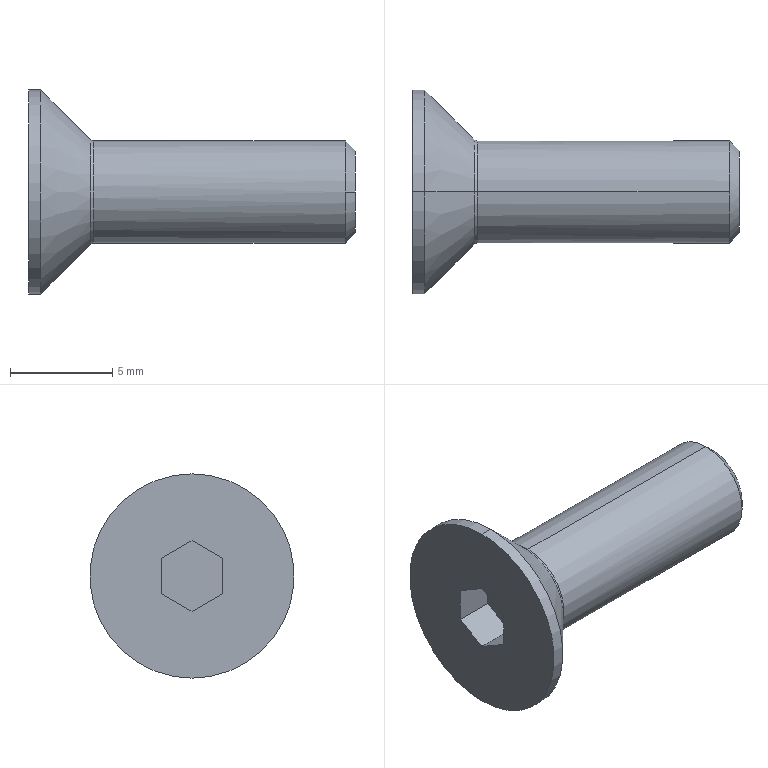Part | STEP file | 1 solid | 19 faces | box 16 x 10 x 10 mm | volume 398.324 mm3 | plane 9 | cylinder 4 | cone 4 | spline 2 | commonest cylinder face diameters 5 x2 10 x2
STEP:
#1=CARTESIAN_POINT('',(0.,0.,0.));
#2=DIRECTION('',(0.,0.,1.));
#3=DIRECTION('',(1.,0.,0.));
#4=AXIS2_PLACEMENT_3D('',#1,#2,#3);
#5=CARTESIAN_POINT('',(-3.1,-1.5,0.866));
#6=VERTEX_POINT('',#5);
#7=CARTESIAN_POINT('',(-1.2,-1.5,0.866));
#8=VERTEX_POINT('',#7);
#9=CARTESIAN_POINT('',(-1.2,-1.5,0.866));
#10=DIRECTION('',(1.,0.,0.));
#11=VECTOR('',#10,1.);
#12=LINE('',#9,#11);
#13=CARTESIAN_POINT('',(-1.2,-1.5,-0.866));
#14=DIRECTION('',(0.,-1.,0.));
#15=DIRECTION('',(-1.,0.,0.));
#16=AXIS2_PLACEMENT_3D('',#13,#14,#15);
#17=PLANE('',#16);
#18=CARTESIAN_POINT('',(0.,-1.732));
#19=DIRECTION('',(-1.,0.));
#20=VECTOR('',#19,1.);
#21=LINE('',#18,#20);
#22=(GEOMETRIC_REPRESENTATION_CONTEXT(2)PARAMETRIC_REPRESENTATION_CONTEXT()REPRESENTATION_CONTEXT('',''));
#23=DEFINITIONAL_REPRESENTATION('',(#21),#22);
#24=PCURVE('',#17,#23);
#25=CARTESIAN_POINT('',(-1.2,-1.5,0.866));
#26=DIRECTION('',(0.,-0.5,0.866));
#27=DIRECTION('',(-1.,0.,0.));
#28=AXIS2_PLACEMENT_3D('',#25,#26,#27);
#29=PLANE('',#28);
#30=CARTESIAN_POINT('',(0.,0.));
#31=DIRECTION('',(-1.,0.));
#32=VECTOR('',#31,1.);
#33=LINE('',#30,#32);
#34=(GEOMETRIC_REPRESENTATION_CONTEXT(2)PARAMETRIC_REPRESENTATION_CONTEXT()REPRESENTATION_CONTEXT('',''));
#35=DEFINITIONAL_REPRESENTATION('',(#33),#34);
#36=PCURVE('',#29,#35);
#37=SURFACE_CURVE('',#12,(#24,#36),.PCURVE_S1.);
#38=EDGE_CURVE('',#6,#8,#37,.T.);
#39=ORIENTED_EDGE('',*,*,#38,.T.);
#40=CARTESIAN_POINT('',(-1.2,-1.5,-0.866));
#41=VERTEX_POINT('',#40);
#42=CARTESIAN_POINT('',(-1.2,-1.5,-0.866));
#43=DIRECTION('',(0.,0.,1.));
#44=VECTOR('',#43,1.);
#45=LINE('',#42,#44);
#46=CARTESIAN_POINT('',(0.,0.));
#47=DIRECTION('',(0.,-1.));
#48=VECTOR('',#47,1.);
#49=LINE('',#46,#48);
#50=(GEOMETRIC_REPRESENTATION_CONTEXT(2)PARAMETRIC_REPRESENTATION_CONTEXT()REPRESENTATION_CONTEXT('',''));
#51=DEFINITIONAL_REPRESENTATION('',(#49),#50);
#52=PCURVE('',#17,#51);
#53=CARTESIAN_POINT('',(-1.2,0.,0.));
#54=DIRECTION('',(-1.,0.,0.));
#55=DIRECTION('',(0.,0.,1.));
#56=AXIS2_PLACEMENT_3D('',#53,#54,#55);
#57=PLANE('',#56);
#58=CARTESIAN_POINT('',(-0.866,-1.5));
#59=DIRECTION('',(1.,0.));
#60=VECTOR('',#59,1.);
#61=LINE('',#58,#60);
#62=(GEOMETRIC_REPRESENTATION_CONTEXT(2)PARAMETRIC_REPRESENTATION_CONTEXT()REPRESENTATION_CONTEXT('',''));
#63=DEFINITIONAL_REPRESENTATION('',(#61),#62);
#64=PCURVE('',#57,#63);
#65=SURFACE_CURVE('',#45,(#52,#64),.PCURVE_S1.);
#66=EDGE_CURVE('',#41,#8,#65,.T.);
#67=ORIENTED_EDGE('',*,*,#66,.F.);
#68=CARTESIAN_POINT('',(-3.1,-1.5,-0.866));
#69=VERTEX_POINT('',#68);
#70=CARTESIAN_POINT('',(-1.2,-1.5,-0.866));
#71=DIRECTION('',(-1.,0.,0.));
#72=VECTOR('',#71,1.);
#73=LINE('',#70,#72);
#74=CARTESIAN_POINT('',(0.,0.));
#75=DIRECTION('',(1.,0.));
#76=VECTOR('',#75,1.);
#77=LINE('',#74,#76);
#78=(GEOMETRIC_REPRESENTATION_CONTEXT(2)PARAMETRIC_REPRESENTATION_CONTEXT()REPRESENTATION_CONTEXT('',''));
#79=DEFINITIONAL_REPRESENTATION('',(#77),#78);
#80=PCURVE('',#17,#79);
#81=CARTESIAN_POINT('',(-1.2,0.,-1.732));
#82=DIRECTION('',(0.,-0.5,-0.866));
#83=DIRECTION('',(0.,-0.866,0.5));
#84=AXIS2_PLACEMENT_3D('',#81,#82,#83);
#85=PLANE('',#84);
#86=CARTESIAN_POINT('',(1.732,0.));
#87=DIRECTION('',(0.,1.));
#88=VECTOR('',#87,1.);
#89=LINE('',#86,#88);
#90=(GEOMETRIC_REPRESENTATION_CONTEXT(2)PARAMETRIC_REPRESENTATION_CONTEXT()REPRESENTATION_CONTEXT('',''));
#91=DEFINITIONAL_REPRESENTATION('',(#89),#90);
#92=PCURVE('',#85,#91);
#93=SURFACE_CURVE('',#73,(#80,#92),.PCURVE_S1.);
#94=EDGE_CURVE('',#41,#69,#93,.T.);
#95=ORIENTED_EDGE('',*,*,#94,.T.);
#96=CARTESIAN_POINT('',(-3.1,-1.5,-0.866));
#97=DIRECTION('',(0.,0.,-1.));
#98=VECTOR('',#97,1.);
#99=LINE('',#96,#98);
#100=CARTESIAN_POINT('',(1.9,0.));
#101=DIRECTION('',(0.,1.));
#102=VECTOR('',#101,1.);
#103=LINE('',#100,#102);
#104=(GEOMETRIC_REPRESENTATION_CONTEXT(2)PARAMETRIC_REPRESENTATION_CONTEXT()REPRESENTATION_CONTEXT('',''));
#105=DEFINITIONAL_REPRESENTATION('',(#103),#104);
#106=PCURVE('',#17,#105);
#107=CARTESIAN_POINT('',(-3.1,5.,0.));
#108=DIRECTION('',(1.,0.,0.));
#109=DIRECTION('',(0.,1.,0.));
#110=AXIS2_PLACEMENT_3D('',#107,#108,#109);
#111=PLANE('',#110);
#112=CARTESIAN_POINT('',(-6.5,-0.866));
#113=DIRECTION('',(0.,-1.));
#114=VECTOR('',#113,1.);
#115=LINE('',#112,#114);
#116=(GEOMETRIC_REPRESENTATION_CONTEXT(2)PARAMETRIC_REPRESENTATION_CONTEXT()REPRESENTATION_CONTEXT('',''));
#117=DEFINITIONAL_REPRESENTATION('',(#115),#116);
#118=PCURVE('',#111,#117);
#119=SURFACE_CURVE('',#99,(#106,#118),.PCURVE_S1.);
#120=EDGE_CURVE('',#6,#69,#119,.T.);
#121=ORIENTED_EDGE('',*,*,#120,.F.);
#122=EDGE_LOOP('',(#39,#67,#95,#121));
#123=FACE_BOUND('',#122,.T.);
#124=ADVANCED_FACE('',(#123),#17,.F.);
#125=CARTESIAN_POINT('',(-3.1,0.,1.732));
#126=VERTEX_POINT('',#125);
#127=CARTESIAN_POINT('',(-1.2,0.,1.732));
#128=VERTEX_POINT('',#127);
#129=CARTESIAN_POINT('',(-1.2,0.,1.732));
#130=DIRECTION('',(1.,0.,0.));
#131=VECTOR('',#130,1.);
#132=LINE('',#129,#131);
#133=CARTESIAN_POINT('',(0.,-1.732));
#134=DIRECTION('',(-1.,0.));
#135=VECTOR('',#134,1.);
#136=LINE('',#133,#135);
#137=(GEOMETRIC_REPRESENTATION_CONTEXT(2)PARAMETRIC_REPRESENTATION_CONTEXT()REPRESENTATION_CONTEXT('',''));
#138=DEFINITIONAL_REPRESENTATION('',(#136),#137);
#139=PCURVE('',#29,#138);
#140=CARTESIAN_POINT('',(-1.2,0.,1.732));
#141=DIRECTION('',(0.,0.5,0.866));
#142=DIRECTION('',(1.,0.,0.));
#143=AXIS2_PLACEMENT_3D('',#140,#141,#142);
#144=PLANE('',#143);
#145=CARTESIAN_POINT('',(0.,0.));
#146=DIRECTION('',(1.,0.));
#147=VECTOR('',#146,1.);
#148=LINE('',#145,#147);
#149=(GEOMETRIC_REPRESENTATION_CONTEXT(2)PARAMETRIC_REPRESENTATION_CONTEXT()REPRESENTATION_CONTEXT('',''));
#150=DEFINITIONAL_REPRESENTATION('',(#148),#149);
#151=PCURVE('',#144,#150);
#152=SURFACE_CURVE('',#132,(#139,#151),.PCURVE_S1.);
#153=EDGE_CURVE('',#126,#128,#152,.T.);
#154=ORIENTED_EDGE('',*,*,#153,.T.);
#155=CARTESIAN_POINT('',(-1.2,-1.5,0.866));
#156=DIRECTION('',(0.,0.866,0.5));
#157=VECTOR('',#156,1.);
#158=LINE('',#155,#157);
#159=CARTESIAN_POINT('',(0.,0.));
#160=DIRECTION('',(0.,-1.));
#161=VECTOR('',#160,1.);
#162=LINE('',#159,#161);
#163=(GEOMETRIC_REPRESENTATION_CONTEXT(2)PARAMETRIC_REPRESENTATION_CONTEXT()REPRESENTATION_CONTEXT('',''));
#164=DEFINITIONAL_REPRESENTATION('',(#162),#163);
#165=PCURVE('',#29,#164);
#166=CARTESIAN_POINT('',(0.866,-1.5));
#167=DIRECTION('',(0.5,0.866));
#168=VECTOR('',#167,1.);
#169=LINE('',#166,#168);
#170=(GEOMETRIC_REPRESENTATION_CONTEXT(2)PARAMETRIC_REPRESENTATION_CONTEXT()REPRESENTATION_CONTEXT('',''));
#171=DEFINITIONAL_REPRESENTATION('',(#169),#170);
#172=PCURVE('',#57,#171);
#173=SURFACE_CURVE('',#158,(#165,#172),.PCURVE_S1.);
#174=EDGE_CURVE('',#8,#128,#173,.T.);
#175=ORIENTED_EDGE('',*,*,#174,.F.);
#176=ORIENTED_EDGE('',*,*,#38,.F.);
#177=CARTESIAN_POINT('',(-3.1,-1.5,0.866));
#178=DIRECTION('',(0.,-0.866,-0.5));
#179=VECTOR('',#178,1.);
#180=LINE('',#177,#179);
#181=CARTESIAN_POINT('',(1.9,0.));
#182=DIRECTION('',(0.,1.));
#183=VECTOR('',#182,1.);
#184=LINE('',#181,#183);
#185=(GEOMETRIC_REPRESENTATION_CONTEXT(2)PARAMETRIC_REPRESENTATION_CONTEXT()REPRESENTATION_CONTEXT('',''));
#186=DEFINITIONAL_REPRESENTATION('',(#184),#185);
#187=PCURVE('',#29,#186);
#188=CARTESIAN_POINT('',(-6.5,0.866));
#189=DIRECTION('',(-0.866,-0.5));
#190=VECTOR('',#189,1.);
#191=LINE('',#188,#190);
#192=(GEOMETRIC_REPRESENTATION_CONTEXT(2)PARAMETRIC_REPRESENTATION_CONTEXT()REPRESENTATION_CONTEXT('',''));
#193=DEFINITIONAL_REPRESENTATION('',(#191),#192);
#194=PCURVE('',#111,#193);
#195=SURFACE_CURVE('',#180,(#187,#194),.PCURVE_S1.);
#196=EDGE_CURVE('',#126,#6,#195,.T.);
#197=ORIENTED_EDGE('',*,*,#196,.F.);
#198=EDGE_LOOP('',(#154,#175,#176,#197));
#199=FACE_BOUND('',#198,.T.);
#200=ADVANCED_FACE('',(#199),#29,.F.);
#201=ORIENTED_EDGE('',*,*,#94,.F.);
#202=CARTESIAN_POINT('',(-1.2,0.,-1.732));
#203=VERTEX_POINT('',#202);
#204=CARTESIAN_POINT('',(-1.2,0.,-1.732));
#205=DIRECTION('',(0.,-0.866,0.5));
#206=VECTOR('',#205,1.);
#207=LINE('',#204,#206);
#208=CARTESIAN_POINT('',(0.,0.));
#209=DIRECTION('',(1.,0.));
#210=VECTOR('',#209,1.);
#211=LINE('',#208,#210);
#212=(GEOMETRIC_REPRESENTATION_CONTEXT(2)PARAMETRIC_REPRESENTATION_CONTEXT()REPRESENTATION_CONTEXT('',''));
#213=DEFINITIONAL_REPRESENTATION('',(#211),#212);
#214=PCURVE('',#85,#213);
#215=CARTESIAN_POINT('',(-1.732,0.));
#216=DIRECTION('',(0.5,-0.866));
#217=VECTOR('',#216,1.);
#218=LINE('',#215,#217);
#219=(GEOMETRIC_REPRESENTATION_CONTEXT(2)PARAMETRIC_REPRESENTATION_CONTEXT()REPRESENTATION_CONTEXT('',''));
#220=DEFINITIONAL_REPRESENTATION('',(#218),#219);
#221=PCURVE('',#57,#220);
#222=SURFACE_CURVE('',#207,(#214,#221),.PCURVE_S1.);
#223=EDGE_CURVE('',#203,#41,#222,.T.);
#224=ORIENTED_EDGE('',*,*,#223,.F.);
#225=CARTESIAN_POINT('',(-3.1,0.,-1.732));
#226=VERTEX_POINT('',#225);
#227=CARTESIAN_POINT('',(-1.2,0.,-1.732));
#228=DIRECTION('',(-1.,0.,0.));
#229=VECTOR('',#228,1.);
#230=LINE('',#227,#229);
#231=CARTESIAN_POINT('',(0.,0.));
#232=DIRECTION('',(0.,1.));
#233=VECTOR('',#232,1.);
#234=LINE('',#231,#233);
#235=(GEOMETRIC_REPRESENTATION_CONTEXT(2)PARAMETRIC_REPRESENTATION_CONTEXT()REPRESENTATION_CONTEXT('',''));
#236=DEFINITIONAL_REPRESENTATION('',(#234),#235);
#237=PCURVE('',#85,#236);
#238=CARTESIAN_POINT('',(-1.2,1.5,-0.866));
#239=DIRECTION('',(0.,0.5,-0.866));
#240=DIRECTION('',(-1.,0.,0.));
#241=AXIS2_PLACEMENT_3D('',#238,#239,#240);
#242=PLANE('',#241);
#243=CARTESIAN_POINT('',(0.,-1.732));
#244=DIRECTION('',(1.,0.));
#245=VECTOR('',#244,1.);
#246=LINE('',#243,#245);
#247=(GEOMETRIC_REPRESENTATION_CONTEXT(2)PARAMETRIC_REPRESENTATION_CONTEXT()REPRESENTATION_CONTEXT('',''));
#248=DEFINITIONAL_REPRESENTATION('',(#246),#247);
#249=PCURVE('',#242,#248);
#250=SURFACE_CURVE('',#230,(#237,#249),.PCURVE_S1.);
#251=EDGE_CURVE('',#203,#226,#250,.T.);
#252=ORIENTED_EDGE('',*,*,#251,.T.);
#253=CARTESIAN_POINT('',(-3.1,0.,-1.732));
#254=DIRECTION('',(0.,0.866,-0.5));
#255=VECTOR('',#254,1.);
#256=LINE('',#253,#255);
#257=CARTESIAN_POINT('',(0.,1.9));
#258=DIRECTION('',(-1.,0.));
#259=VECTOR('',#258,1.);
#260=LINE('',#257,#259);
#261=(GEOMETRIC_REPRESENTATION_CONTEXT(2)PARAMETRIC_REPRESENTATION_CONTEXT()REPRESENTATION_CONTEXT('',''));
#262=DEFINITIONAL_REPRESENTATION('',(#260),#261);
#263=PCURVE('',#85,#262);
#264=CARTESIAN_POINT('',(-5.,-1.732));
#265=DIRECTION('',(0.866,-0.5));
#266=VECTOR('',#265,1.);
#267=LINE('',#264,#266);
#268=(GEOMETRIC_REPRESENTATION_CONTEXT(2)PARAMETRIC_REPRESENTATION_CONTEXT()REPRESENTATION_CONTEXT('',''));
#269=DEFINITIONAL_REPRESENTATION('',(#267),#268);
#270=PCURVE('',#111,#269);
#271=SURFACE_CURVE('',#256,(#263,#270),.PCURVE_S1.);
#272=EDGE_CURVE('',#69,#226,#271,.T.);
#273=ORIENTED_EDGE('',*,*,#272,.F.);
#274=EDGE_LOOP('',(#201,#224,#252,#273));
#275=FACE_BOUND('',#274,.T.);
#276=ADVANCED_FACE('',(#275),#85,.F.);
#277=CARTESIAN_POINT('',(-3.1,1.5,0.866));
#278=VERTEX_POINT('',#277);
#279=CARTESIAN_POINT('',(-1.2,1.5,0.866));
#280=VERTEX_POINT('',#279);
#281=CARTESIAN_POINT('',(-1.2,1.5,0.866));
#282=DIRECTION('',(1.,0.,0.));
#283=VECTOR('',#282,1.);
#284=LINE('',#281,#283);
#285=CARTESIAN_POINT('',(0.,1.732));
#286=DIRECTION('',(1.,0.));
#287=VECTOR('',#286,1.);
#288=LINE('',#285,#287);
#289=(GEOMETRIC_REPRESENTATION_CONTEXT(2)PARAMETRIC_REPRESENTATION_CONTEXT()REPRESENTATION_CONTEXT('',''));
#290=DEFINITIONAL_REPRESENTATION('',(#288),#289);
#291=PCURVE('',#144,#290);
#292=CARTESIAN_POINT('',(-1.2,1.5,0.866));
#293=DIRECTION('',(0.,1.,0.));
#294=DIRECTION('',(1.,0.,0.));
#295=AXIS2_PLACEMENT_3D('',#292,#293,#294);
#296=PLANE('',#295);
#297=CARTESIAN_POINT('',(0.,0.));
#298=DIRECTION('',(1.,0.));
#299=VECTOR('',#298,1.);
#300=LINE('',#297,#299);
#301=(GEOMETRIC_REPRESENTATION_CONTEXT(2)PARAMETRIC_REPRESENTATION_CONTEXT()REPRESENTATION_CONTEXT('',''));
#302=DEFINITIONAL_REPRESENTATION('',(#300),#301);
#303=PCURVE('',#296,#302);
#304=SURFACE_CURVE('',#284,(#291,#303),.PCURVE_S1.);
#305=EDGE_CURVE('',#278,#280,#304,.T.);
#306=ORIENTED_EDGE('',*,*,#305,.T.);
#307=CARTESIAN_POINT('',(-1.2,0.,1.732));
#308=DIRECTION('',(0.,0.866,-0.5));
#309=VECTOR('',#308,1.);
#310=LINE('',#307,#309);
#311=CARTESIAN_POINT('',(0.,0.));
#312=DIRECTION('',(0.,1.));
#313=VECTOR('',#312,1.);
#314=LINE('',#311,#313);
#315=(GEOMETRIC_REPRESENTATION_CONTEXT(2)PARAMETRIC_REPRESENTATION_CONTEXT()REPRESENTATION_CONTEXT('',''));
#316=DEFINITIONAL_REPRESENTATION('',(#314),#315);
#317=PCURVE('',#144,#316);
#318=CARTESIAN_POINT('',(1.732,0.));
#319=DIRECTION('',(-0.5,0.866));
#320=VECTOR('',#319,1.);
#321=LINE('',#318,#320);
#322=(GEOMETRIC_REPRESENTATION_CONTEXT(2)PARAMETRIC_REPRESENTATION_CONTEXT()REPRESENTATION_CONTEXT('',''));
#323=DEFINITIONAL_REPRESENTATION('',(#321),#322);
#324=PCURVE('',#57,#323);
#325=SURFACE_CURVE('',#310,(#317,#324),.PCURVE_S1.);
#326=EDGE_CURVE('',#128,#280,#325,.T.);
#327=ORIENTED_EDGE('',*,*,#326,.F.);
#328=ORIENTED_EDGE('',*,*,#153,.F.);
#329=CARTESIAN_POINT('',(-3.1,0.,1.732));
#330=DIRECTION('',(0.,-0.866,0.5));
#331=VECTOR('',#330,1.);
#332=LINE('',#329,#331);
#333=CARTESIAN_POINT('',(-1.9,0.));
#334=DIRECTION('',(0.,-1.));
#335=VECTOR('',#334,1.);
#336=LINE('',#333,#335);
#337=(GEOMETRIC_REPRESENTATION_CONTEXT(2)PARAMETRIC_REPRESENTATION_CONTEXT()REPRESENTATION_CONTEXT('',''));
#338=DEFINITIONAL_REPRESENTATION('',(#336),#337);
#339=PCURVE('',#144,#338);
#340=CARTESIAN_POINT('',(-5.,1.732));
#341=DIRECTION('',(-0.866,0.5));
#342=VECTOR('',#341,1.);
#343=LINE('',#340,#342);
#344=(GEOMETRIC_REPRESENTATION_CONTEXT(2)PARAMETRIC_REPRESENTATION_CONTEXT()REPRESENTATION_CONTEXT('',''));
#345=DEFINITIONAL_REPRESENTATION('',(#343),#344);
#346=PCURVE('',#111,#345);
#347=SURFACE_CURVE('',#332,(#339,#346),.PCURVE_S1.);
#348=EDGE_CURVE('',#278,#126,#347,.T.);
#349=ORIENTED_EDGE('',*,*,#348,.F.);
#350=EDGE_LOOP('',(#306,#327,#328,#349));
#351=FACE_BOUND('',#350,.T.);
#352=ADVANCED_FACE('',(#351),#144,.F.);
#353=ORIENTED_EDGE('',*,*,#66,.T.);
#354=ORIENTED_EDGE('',*,*,#174,.T.);
#355=ORIENTED_EDGE('',*,*,#326,.T.);
#356=CARTESIAN_POINT('',(-1.2,1.5,-0.866));
#357=VERTEX_POINT('',#356);
#358=CARTESIAN_POINT('',(-1.2,1.5,0.866));
#359=DIRECTION('',(0.,0.,-1.));
#360=VECTOR('',#359,1.);
#361=LINE('',#358,#360);
#362=CARTESIAN_POINT('',(0.866,1.5));
#363=DIRECTION('',(-1.,0.));
#364=VECTOR('',#363,1.);
#365=LINE('',#362,#364);
#366=(GEOMETRIC_REPRESENTATION_CONTEXT(2)PARAMETRIC_REPRESENTATION_CONTEXT()REPRESENTATION_CONTEXT('',''));
#367=DEFINITIONAL_REPRESENTATION('',(#365),#366);
#368=PCURVE('',#57,#367);
#369=CARTESIAN_POINT('',(0.,0.));
#370=DIRECTION('',(0.,1.));
#371=VECTOR('',#370,1.);
#372=LINE('',#369,#371);
#373=(GEOMETRIC_REPRESENTATION_CONTEXT(2)PARAMETRIC_REPRESENTATION_CONTEXT()REPRESENTATION_CONTEXT('',''));
#374=DEFINITIONAL_REPRESENTATION('',(#372),#373);
#375=PCURVE('',#296,#374);
#376=SURFACE_CURVE('',#361,(#368,#375),.PCURVE_S1.);
#377=EDGE_CURVE('',#280,#357,#376,.T.);
#378=ORIENTED_EDGE('',*,*,#377,.T.);
#379=CARTESIAN_POINT('',(-1.2,1.5,-0.866));
#380=DIRECTION('',(0.,-0.866,-0.5));
#381=VECTOR('',#380,1.);
#382=LINE('',#379,#381);
#383=CARTESIAN_POINT('',(-0.866,1.5));
#384=DIRECTION('',(-0.5,-0.866));
#385=VECTOR('',#384,1.);
#386=LINE('',#383,#385);
#387=(GEOMETRIC_REPRESENTATION_CONTEXT(2)PARAMETRIC_REPRESENTATION_CONTEXT()REPRESENTATION_CONTEXT('',''));
#388=DEFINITIONAL_REPRESENTATION('',(#386),#387);
#389=PCURVE('',#57,#388);
#390=CARTESIAN_POINT('',(0.,0.));
#391=DIRECTION('',(0.,-1.));
#392=VECTOR('',#391,1.);
#393=LINE('',#390,#392);
#394=(GEOMETRIC_REPRESENTATION_CONTEXT(2)PARAMETRIC_REPRESENTATION_CONTEXT()REPRESENTATION_CONTEXT('',''));
#395=DEFINITIONAL_REPRESENTATION('',(#393),#394);
#396=PCURVE('',#242,#395);
#397=SURFACE_CURVE('',#382,(#389,#396),.PCURVE_S1.);
#398=EDGE_CURVE('',#357,#203,#397,.T.);
#399=ORIENTED_EDGE('',*,*,#398,.T.);
#400=ORIENTED_EDGE('',*,*,#223,.T.);
#401=EDGE_LOOP('',(#353,#354,#355,#378,#399,#400));
#402=FACE_BOUND('',#401,.T.);
#403=ADVANCED_FACE('',(#402),#57,.T.);
#404=ORIENTED_EDGE('',*,*,#251,.F.);
#405=ORIENTED_EDGE('',*,*,#398,.F.);
#406=CARTESIAN_POINT('',(-3.1,1.5,-0.866));
#407=VERTEX_POINT('',#406);
#408=CARTESIAN_POINT('',(-1.2,1.5,-0.866));
#409=DIRECTION('',(-1.,0.,0.));
#410=VECTOR('',#409,1.);
#411=LINE('',#408,#410);
#412=CARTESIAN_POINT('',(0.,0.));
#413=DIRECTION('',(1.,0.));
#414=VECTOR('',#413,1.);
#415=LINE('',#412,#414);
#416=(GEOMETRIC_REPRESENTATION_CONTEXT(2)PARAMETRIC_REPRESENTATION_CONTEXT()REPRESENTATION_CONTEXT('',''));
#417=DEFINITIONAL_REPRESENTATION('',(#415),#416);
#418=PCURVE('',#242,#417);
#419=CARTESIAN_POINT('',(0.,1.732));
#420=DIRECTION('',(-1.,0.));
#421=VECTOR('',#420,1.);
#422=LINE('',#419,#421);
#423=(GEOMETRIC_REPRESENTATION_CONTEXT(2)PARAMETRIC_REPRESENTATION_CONTEXT()REPRESENTATION_CONTEXT('',''));
#424=DEFINITIONAL_REPRESENTATION('',(#422),#423);
#425=PCURVE('',#296,#424);
#426=SURFACE_CURVE('',#411,(#418,#425),.PCURVE_S1.);
#427=EDGE_CURVE('',#357,#407,#426,.T.);
#428=ORIENTED_EDGE('',*,*,#427,.T.);
#429=CARTESIAN_POINT('',(-3.1,1.5,-0.866));
#430=DIRECTION('',(0.,0.866,0.5));
#431=VECTOR('',#430,1.);
#432=LINE('',#429,#431);
#433=CARTESIAN_POINT('',(1.9,0.));
#434=DIRECTION('',(0.,1.));
#435=VECTOR('',#434,1.);
#436=LINE('',#433,#435);
#437=(GEOMETRIC_REPRESENTATION_CONTEXT(2)PARAMETRIC_REPRESENTATION_CONTEXT()REPRESENTATION_CONTEXT('',''));
#438=DEFINITIONAL_REPRESENTATION('',(#436),#437);
#439=PCURVE('',#242,#438);
#440=CARTESIAN_POINT('',(-3.5,-0.866));
#441=DIRECTION('',(0.866,0.5));
#442=VECTOR('',#441,1.);
#443=LINE('',#440,#442);
#444=(GEOMETRIC_REPRESENTATION_CONTEXT(2)PARAMETRIC_REPRESENTATION_CONTEXT()REPRESENTATION_CONTEXT('',''));
#445=DEFINITIONAL_REPRESENTATION('',(#443),#444);
#446=PCURVE('',#111,#445);
#447=SURFACE_CURVE('',#432,(#439,#446),.PCURVE_S1.);
#448=EDGE_CURVE('',#226,#407,#447,.T.);
#449=ORIENTED_EDGE('',*,*,#448,.F.);
#450=EDGE_LOOP('',(#404,#405,#428,#449));
#451=FACE_BOUND('',#450,.T.);
#452=ADVANCED_FACE('',(#451),#242,.F.);
#453=ORIENTED_EDGE('',*,*,#427,.F.);
#454=ORIENTED_EDGE('',*,*,#377,.F.);
#455=ORIENTED_EDGE('',*,*,#305,.F.);
#456=CARTESIAN_POINT('',(-3.1,1.5,0.));
#457=DIRECTION('',(0.,0.,-1.));
#458=VECTOR('',#457,1.);
#459=LINE('',#456,#458);
#460=CARTESIAN_POINT('',(-1.9,0.866));
#461=DIRECTION('',(0.,1.));
#462=VECTOR('',#461,1.);
#463=LINE('',#460,#462);
#464=(GEOMETRIC_REPRESENTATION_CONTEXT(2)PARAMETRIC_REPRESENTATION_CONTEXT()REPRESENTATION_CONTEXT('',''));
#465=DEFINITIONAL_REPRESENTATION('',(#463),#464);
#466=PCURVE('',#296,#465);
#467=CARTESIAN_POINT('',(-3.5,0.));
#468=DIRECTION('',(0.,-1.));
#469=VECTOR('',#468,1.);
#470=LINE('',#467,#469);
#471=(GEOMETRIC_REPRESENTATION_CONTEXT(2)PARAMETRIC_REPRESENTATION_CONTEXT()REPRESENTATION_CONTEXT('',''));
#472=DEFINITIONAL_REPRESENTATION('',(#470),#471);
#473=PCURVE('',#111,#472);
#474=SURFACE_CURVE('',#459,(#466,#473),.PCURVE_S1.);
#475=EDGE_CURVE('',#278,#407,#474,.T.);
#476=ORIENTED_EDGE('',*,*,#475,.T.);
#477=EDGE_LOOP('',(#453,#454,#455,#476));
#478=FACE_BOUND('',#477,.T.);
#479=ADVANCED_FACE('',(#478),#296,.F.);
#480=ORIENTED_EDGE('',*,*,#348,.T.);
#481=ORIENTED_EDGE('',*,*,#196,.T.);
#482=ORIENTED_EDGE('',*,*,#120,.T.);
#483=ORIENTED_EDGE('',*,*,#272,.T.);
#484=ORIENTED_EDGE('',*,*,#448,.T.);
#485=ORIENTED_EDGE('',*,*,#475,.F.);
#486=EDGE_LOOP('',(#480,#481,#482,#483,#484,#485));
#487=FACE_BOUND('',#486,.T.);
#488=CARTESIAN_POINT('',(-3.1,0.,5.));
#489=VERTEX_POINT('',#488);
#490=CARTESIAN_POINT('',(-3.1,0.,-5.));
#491=VERTEX_POINT('',#490);
#492=CARTESIAN_POINT('',(-3.1,0.,0.));
#493=DIRECTION('',(1.,0.,0.));
#494=DIRECTION('',(0.,0.,1.));
#495=AXIS2_PLACEMENT_3D('',#492,#493,#494);
#496=CIRCLE('',#495,5.);
#497=CARTESIAN_POINT('',(-5.,0.));
#498=DIRECTION('',(0.,1.));
#499=AXIS2_PLACEMENT_2D('',#497,#498);
#500=CIRCLE('',#499,5.);
#501=(GEOMETRIC_REPRESENTATION_CONTEXT(2)PARAMETRIC_REPRESENTATION_CONTEXT()REPRESENTATION_CONTEXT('',''));
#502=DEFINITIONAL_REPRESENTATION('',(#500),#501);
#503=PCURVE('',#111,#502);
#504=CARTESIAN_POINT('',(-20.912,0.,0.));
#505=DIRECTION('',(-1.,0.,0.));
#506=DIRECTION('',(0.,0.,1.));
#507=AXIS2_PLACEMENT_3D('',#504,#505,#506);
#508=CYLINDRICAL_SURFACE('',#507,5.);
#509=CARTESIAN_POINT('',(6.283,-17.812));
#510=DIRECTION('',(-1.,0.));
#511=VECTOR('',#510,1.);
#512=LINE('',#509,#511);
#513=(GEOMETRIC_REPRESENTATION_CONTEXT(2)PARAMETRIC_REPRESENTATION_CONTEXT()REPRESENTATION_CONTEXT('',''));
#514=DEFINITIONAL_REPRESENTATION('',(#512),#513);
#515=PCURVE('',#508,#514);
#516=SURFACE_CURVE('',#496,(#503,#515),.PCURVE_S1.);
#517=EDGE_CURVE('',#489,#491,#516,.T.);
#518=ORIENTED_EDGE('',*,*,#517,.F.);
#519=CARTESIAN_POINT('',(-3.1,0.,0.));
#520=DIRECTION('',(1.,0.,0.));
#521=DIRECTION('',(0.,0.,1.));
#522=AXIS2_PLACEMENT_3D('',#519,#520,#521);
#523=CIRCLE('',#522,5.);
#524=CARTESIAN_POINT('',(-5.,0.));
#525=DIRECTION('',(0.,1.));
#526=AXIS2_PLACEMENT_2D('',#524,#525);
#527=CIRCLE('',#526,5.);
#528=(GEOMETRIC_REPRESENTATION_CONTEXT(2)PARAMETRIC_REPRESENTATION_CONTEXT()REPRESENTATION_CONTEXT('',''));
#529=DEFINITIONAL_REPRESENTATION('',(#527),#528);
#530=PCURVE('',#111,#529);
#531=CARTESIAN_POINT('',(-20.912,0.,0.));
#532=DIRECTION('',(-1.,0.,0.));
#533=DIRECTION('',(0.,0.,1.));
#534=AXIS2_PLACEMENT_3D('',#531,#532,#533);
#535=CYLINDRICAL_SURFACE('',#534,5.);
#536=CARTESIAN_POINT('',(6.283,-17.812));
#537=DIRECTION('',(-1.,0.));
#538=VECTOR('',#537,1.);
#539=LINE('',#536,#538);
#540=(GEOMETRIC_REPRESENTATION_CONTEXT(2)PARAMETRIC_REPRESENTATION_CONTEXT()REPRESENTATION_CONTEXT('',''));
#541=DEFINITIONAL_REPRESENTATION('',(#539),#540);
#542=PCURVE('',#535,#541);
#543=SURFACE_CURVE('',#523,(#530,#542),.PCURVE_S1.);
#544=EDGE_CURVE('',#491,#489,#543,.T.);
#545=ORIENTED_EDGE('',*,*,#544,.F.);
#546=EDGE_LOOP('',(#518,#545));
#547=FACE_BOUND('',#546,.T.);
#548=ADVANCED_FACE('',(#487,#547),#111,.F.);
#549=CARTESIAN_POINT('',(-2.5,0.,-5.));
#550=VERTEX_POINT('',#549);
#551=CARTESIAN_POINT('',(-20.912,0.,-5.));
#552=DIRECTION('',(-1.,0.,0.));
#553=VECTOR('',#552,1.);
#554=LINE('',#551,#553);
#555=CARTESIAN_POINT('',(3.142,0.));
#556=DIRECTION('',(0.,1.));
#557=VECTOR('',#556,1.);
#558=LINE('',#555,#557);
#559=(GEOMETRIC_REPRESENTATION_CONTEXT(2)PARAMETRIC_REPRESENTATION_CONTEXT()REPRESENTATION_CONTEXT('',''));
#560=DEFINITIONAL_REPRESENTATION('',(#558),#559);
#561=PCURVE('',#508,#560);
#562=CARTESIAN_POINT('',(3.142,0.));
#563=DIRECTION('',(0.,1.));
#564=VECTOR('',#563,1.);
#565=LINE('',#562,#564);
#566=(GEOMETRIC_REPRESENTATION_CONTEXT(2)PARAMETRIC_REPRESENTATION_CONTEXT()REPRESENTATION_CONTEXT('',''));
#567=DEFINITIONAL_REPRESENTATION('',(#565),#566);
#568=PCURVE('',#535,#567);
#569=SURFACE_CURVE('',#554,(#561,#568),.PCURVE_S1.);
#570=EDGE_CURVE('',#550,#491,#569,.T.);
#571=ORIENTED_EDGE('',*,*,#570,.F.);
#572=CARTESIAN_POINT('',(-2.5,0.,5.));
#573=VERTEX_POINT('',#572);
#574=CARTESIAN_POINT('',(-2.5,0.,0.));
#575=DIRECTION('',(1.,0.,0.));
#576=DIRECTION('',(0.,0.,1.));
#577=AXIS2_PLACEMENT_3D('',#574,#575,#576);
#578=CIRCLE('',#577,5.);
#579=CARTESIAN_POINT('',(6.283,-18.412));
#580=DIRECTION('',(-1.,0.));
#581=VECTOR('',#580,1.);
#582=LINE('',#579,#581);
#583=(GEOMETRIC_REPRESENTATION_CONTEXT(2)PARAMETRIC_REPRESENTATION_CONTEXT()REPRESENTATION_CONTEXT('',''));
#584=DEFINITIONAL_REPRESENTATION('',(#582),#583);
#585=PCURVE('',#508,#584);
#586=CARTESIAN_POINT('',(-2.5,0.,0.));
#587=DIRECTION('',(-1.,0.,0.));
#588=DIRECTION('',(0.,0.,1.));
#589=AXIS2_PLACEMENT_3D('',#586,#587,#588);
#590=CONICAL_SURFACE('',#589,5.,0.7854);
#591=CARTESIAN_POINT('',(6.283,0.));
#592=DIRECTION('',(-1.,0.));
#593=VECTOR('',#592,1.);
#594=LINE('',#591,#593);
#595=(GEOMETRIC_REPRESENTATION_CONTEXT(2)PARAMETRIC_REPRESENTATION_CONTEXT()REPRESENTATION_CONTEXT('',''));
#596=DEFINITIONAL_REPRESENTATION('',(#594),#595);
#597=PCURVE('',#590,#596);
#598=SURFACE_CURVE('',#578,(#585,#597),.PCURVE_S1.);
#599=EDGE_CURVE('',#573,#550,#598,.T.);
#600=ORIENTED_EDGE('',*,*,#599,.F.);
#601=CARTESIAN_POINT('',(-20.912,0.,5.));
#602=DIRECTION('',(-1.,0.,0.));
#603=VECTOR('',#602,1.);
#604=LINE('',#601,#603);
#605=CARTESIAN_POINT('',(6.283,0.));
#606=DIRECTION('',(0.,1.));
#607=VECTOR('',#606,1.);
#608=LINE('',#605,#607);
#609=(GEOMETRIC_REPRESENTATION_CONTEXT(2)PARAMETRIC_REPRESENTATION_CONTEXT()REPRESENTATION_CONTEXT('',''));
#610=DEFINITIONAL_REPRESENTATION('',(#608),#609);
#611=PCURVE('',#508,#610);
#612=CARTESIAN_POINT('',(0.,0.));
#613=DIRECTION('',(0.,1.));
#614=VECTOR('',#613,1.);
#615=LINE('',#612,#614);
#616=(GEOMETRIC_REPRESENTATION_CONTEXT(2)PARAMETRIC_REPRESENTATION_CONTEXT()REPRESENTATION_CONTEXT('',''));
#617=DEFINITIONAL_REPRESENTATION('',(#615),#616);
#618=PCURVE('',#535,#617);
#619=SURFACE_CURVE('',#604,(#611,#618),.PCURVE_S1.);
#620=EDGE_CURVE('',#573,#489,#619,.T.);
#621=ORIENTED_EDGE('',*,*,#620,.T.);
#622=ORIENTED_EDGE('',*,*,#517,.T.);
#623=EDGE_LOOP('',(#571,#600,#621,#622));
#624=FACE_BOUND('',#623,.T.);
#625=ADVANCED_FACE('',(#624),#508,.T.);
#626=CARTESIAN_POINT('',(12.9,-2.,0.));
#627=VERTEX_POINT('',#626);
#628=CARTESIAN_POINT('',(12.9,2.,0.));
#629=VERTEX_POINT('',#628);
#630=CARTESIAN_POINT('',(12.9,0.,0.));
#631=DIRECTION('',(-1.,0.,0.));
#632=DIRECTION('',(0.,-1.,0.));
#633=AXIS2_PLACEMENT_3D('',#630,#631,#632);
#634=CIRCLE('',#633,2.);
#635=CARTESIAN_POINT('',(12.9,2.5,0.));
#636=DIRECTION('',(-1.,0.,0.));
#637=DIRECTION('',(0.,0.,1.));
#638=AXIS2_PLACEMENT_3D('',#635,#636,#637);
#639=PLANE('',#638);
#640=CARTESIAN_POINT('',(0.,-2.5));
#641=DIRECTION('',(0.,-1.));
#642=AXIS2_PLACEMENT_2D('',#640,#641);
#643=CIRCLE('',#642,2.);
#644=(GEOMETRIC_REPRESENTATION_CONTEXT(2)PARAMETRIC_REPRESENTATION_CONTEXT()REPRESENTATION_CONTEXT('',''));
#645=DEFINITIONAL_REPRESENTATION('',(#643),#644);
#646=PCURVE('',#639,#645);
#647=CARTESIAN_POINT('',(12.4,0.,0.));
#648=DIRECTION('',(-1.,0.,0.));
#649=DIRECTION('',(0.,-1.,0.));
#650=AXIS2_PLACEMENT_3D('',#647,#648,#649);
#651=CONICAL_SURFACE('',#650,2.5,0.7854);
#652=CARTESIAN_POINT('',(0.,-0.5));
#653=DIRECTION('',(1.,0.));
#654=VECTOR('',#653,1.);
#655=LINE('',#652,#654);
#656=(GEOMETRIC_REPRESENTATION_CONTEXT(2)PARAMETRIC_REPRESENTATION_CONTEXT()REPRESENTATION_CONTEXT('',''));
#657=DEFINITIONAL_REPRESENTATION('',(#655),#656);
#658=PCURVE('',#651,#657);
#659=SURFACE_CURVE('',#634,(#646,#658),.PCURVE_S1.);
#660=EDGE_CURVE('',#627,#629,#659,.T.);
#661=ORIENTED_EDGE('',*,*,#660,.F.);
#662=CARTESIAN_POINT('',(12.9,0.,0.));
#663=DIRECTION('',(-1.,0.,0.));
#664=DIRECTION('',(0.,-1.,0.));
#665=AXIS2_PLACEMENT_3D('',#662,#663,#664);
#666=CIRCLE('',#665,2.);
#667=CARTESIAN_POINT('',(0.,-2.5));
#668=DIRECTION('',(0.,-1.));
#669=AXIS2_PLACEMENT_2D('',#667,#668);
#670=CIRCLE('',#669,2.);
#671=(GEOMETRIC_REPRESENTATION_CONTEXT(2)PARAMETRIC_REPRESENTATION_CONTEXT()REPRESENTATION_CONTEXT('',''));
#672=DEFINITIONAL_REPRESENTATION('',(#670),#671);
#673=PCURVE('',#639,#672);
#674=CARTESIAN_POINT('',(12.4,0.,0.));
#675=DIRECTION('',(-1.,0.,0.));
#676=DIRECTION('',(0.,-1.,0.));
#677=AXIS2_PLACEMENT_3D('',#674,#675,#676);
#678=CONICAL_SURFACE('',#677,2.5,0.7854);
#679=CARTESIAN_POINT('',(0.,-0.5));
#680=DIRECTION('',(1.,0.));
#681=VECTOR('',#680,1.);
#682=LINE('',#679,#681);
#683=(GEOMETRIC_REPRESENTATION_CONTEXT(2)PARAMETRIC_REPRESENTATION_CONTEXT()REPRESENTATION_CONTEXT('',''));
#684=DEFINITIONAL_REPRESENTATION('',(#682),#683);
#685=PCURVE('',#678,#684);
#686=SURFACE_CURVE('',#666,(#673,#685),.PCURVE_S1.);
#687=EDGE_CURVE('',#629,#627,#686,.T.);
#688=ORIENTED_EDGE('',*,*,#687,.F.);
#689=EDGE_LOOP('',(#661,#688));
#690=FACE_BOUND('',#689,.T.);
#691=ADVANCED_FACE('',(#690),#639,.F.);
#692=CARTESIAN_POINT('',(-0.05858,0.,-2.559));
#693=VERTEX_POINT('',#692);
#694=CARTESIAN_POINT('',(-2.5,0.,-5.));
#695=DIRECTION('',(-0.7071,0.,-0.7071));
#696=VECTOR('',#695,1.);
#697=LINE('',#694,#696);
#698=CARTESIAN_POINT('',(3.142,0.));
#699=DIRECTION('',(0.,1.));
#700=VECTOR('',#699,1.);
#701=LINE('',#698,#700);
#702=(GEOMETRIC_REPRESENTATION_CONTEXT(2)PARAMETRIC_REPRESENTATION_CONTEXT()REPRESENTATION_CONTEXT('',''));
#703=DEFINITIONAL_REPRESENTATION('',(#701),#702);
#704=PCURVE('',#590,#703);
#705=CARTESIAN_POINT('',(-2.5,0.,0.));
#706=DIRECTION('',(-1.,0.,0.));
#707=DIRECTION('',(0.,0.,1.));
#708=AXIS2_PLACEMENT_3D('',#705,#706,#707);
#709=CONICAL_SURFACE('',#708,5.,0.7854);
#710=CARTESIAN_POINT('',(3.142,0.));
#711=DIRECTION('',(0.,1.));
#712=VECTOR('',#711,1.);
#713=LINE('',#710,#712);
#714=(GEOMETRIC_REPRESENTATION_CONTEXT(2)PARAMETRIC_REPRESENTATION_CONTEXT()REPRESENTATION_CONTEXT('',''));
#715=DEFINITIONAL_REPRESENTATION('',(#713),#714);
#716=PCURVE('',#709,#715);
#717=SURFACE_CURVE('',#697,(#704,#716),.PCURVE_S1.);
#718=EDGE_CURVE('',#693,#550,#717,.T.);
#719=ORIENTED_EDGE('',*,*,#718,.F.);
#720=CARTESIAN_POINT('',(-0.05858,0.,2.559));
#721=VERTEX_POINT('',#720);
#722=CARTESIAN_POINT('',(-0.05858,0.,0.));
#723=DIRECTION('',(-1.,0.,0.));
#724=DIRECTION('',(0.,0.,1.));
#725=AXIS2_PLACEMENT_3D('',#722,#723,#724);
#726=CIRCLE('',#725,2.559);
#727=CARTESIAN_POINT('',(0.,-2.441));
#728=DIRECTION('',(1.,0.));
#729=VECTOR('',#728,1.);
#730=LINE('',#727,#729);
#731=(GEOMETRIC_REPRESENTATION_CONTEXT(2)PARAMETRIC_REPRESENTATION_CONTEXT()REPRESENTATION_CONTEXT('',''));
#732=DEFINITIONAL_REPRESENTATION('',(#730),#731);
#733=PCURVE('',#590,#732);
#734=CARTESIAN_POINT('',(0.08284,0.,-2.5));
#735=CARTESIAN_POINT('',(0.08284,-5.,-2.5));
#736=CARTESIAN_POINT('',(0.08284,-5.,2.5));
#737=CARTESIAN_POINT('',(0.08284,0.,2.5));
#738=CARTESIAN_POINT('',(0.02909,0.,-2.5));
#739=CARTESIAN_POINT('',(0.02909,-5.,-2.5));
#740=CARTESIAN_POINT('',(0.02909,-5.,2.5));
#741=CARTESIAN_POINT('',(0.02909,0.,2.5));
#742=CARTESIAN_POINT('',(-0.02057,0.,-2.521));
#743=CARTESIAN_POINT('',(-0.02057,-5.041,-2.521));
#744=CARTESIAN_POINT('',(-0.02057,-5.041,2.521));
#745=CARTESIAN_POINT('',(-0.02057,0.,2.521));
#746=CARTESIAN_POINT('',(-0.05858,0.,-2.559));
#747=CARTESIAN_POINT('',(-0.05858,-5.117,-2.559));
#748=CARTESIAN_POINT('',(-0.05858,-5.117,2.559));
#749=CARTESIAN_POINT('',(-0.05858,0.,2.559));
#750=(BOUNDED_SURFACE()B_SPLINE_SURFACE(3,3,((#734,#735,#736,#737),(#738,#739,#740,#741),(#742,#743,#744,#745),(#746,#747,#748,#749)),.UNSPECIFIED.,.F.,.F.,.F.)B_SPLINE_SURFACE_WITH_KNOTS((4,4),(4,4),(0.,1.),(0.,1.),.PIECEWISE_BEZIER_KNOTS.)GEOMETRIC_REPRESENTATION_ITEM()RATIONAL_B_SPLINE_SURFACE(((1.,0.3333,0.3333,1.),(0.9493,0.3164,0.3164,0.9493),(0.9493,0.3164,0.3164,0.9493),(1.,0.3333,0.3333,1.)))REPRESENTATION_ITEM('')SURFACE());
#751=CARTESIAN_POINT('',(1.,0.));
#752=CARTESIAN_POINT('',(1.,0.02375));
#753=CARTESIAN_POINT('',(1.,0.06805));
#754=CARTESIAN_POINT('',(1.,0.1267));
#755=CARTESIAN_POINT('',(1.,0.1794));
#756=CARTESIAN_POINT('',(1.,0.2276));
#757=CARTESIAN_POINT('',(1.,0.2721));
#758=CARTESIAN_POINT('',(1.,0.3139));
#759=CARTESIAN_POINT('',(1.,0.3535));
#760=CARTESIAN_POINT('',(1.,0.3914));
#761=CARTESIAN_POINT('',(1.,0.4282));
#762=CARTESIAN_POINT('',(1.,0.4643));
#763=CARTESIAN_POINT('',(1.,0.5));
#764=CARTESIAN_POINT('',(1.,0.5357));
#765=CARTESIAN_POINT('',(1.,0.5718));
#766=CARTESIAN_POINT('',(1.,0.6086));
#767=CARTESIAN_POINT('',(1.,0.6465));
#768=CARTESIAN_POINT('',(1.,0.6861));
#769=CARTESIAN_POINT('',(1.,0.7279));
#770=CARTESIAN_POINT('',(1.,0.7724));
#771=CARTESIAN_POINT('',(1.,0.8206));
#772=CARTESIAN_POINT('',(1.,0.8733));
#773=CARTESIAN_POINT('',(1.,0.9319));
#774=CARTESIAN_POINT('',(1.,0.9763));
#775=CARTESIAN_POINT('',(1.,1.));
#776=B_SPLINE_CURVE_WITH_KNOTS('',3,(#751,#752,#753,#754,#755,#756,#757,#758,#759,#760,#761,#762,#763,#764,#765,#766,#767,#768,#769,#770,#771,#772,#773,#774,#775),.UNSPECIFIED.,.F.,.F.,(4,1,1,1,1,1,1,1,1,1,1,1,1,1,1,1,1,1,1,1,1,1,4),(3.142,3.284,3.427,3.57,3.713,3.856,3.998,4.141,4.284,4.427,4.57,4.712,4.855,4.998,5.141,5.284,5.426,5.569,5.712,5.855,5.998,6.14,6.283),.QUASI_UNIFORM_KNOTS.);
#777=(GEOMETRIC_REPRESENTATION_CONTEXT(2)PARAMETRIC_REPRESENTATION_CONTEXT()REPRESENTATION_CONTEXT('',''));
#778=DEFINITIONAL_REPRESENTATION('',(#776),#777);
#779=PCURVE('',#750,#778);
#780=SURFACE_CURVE('',#726,(#733,#779),.PCURVE_S1.);
#781=EDGE_CURVE('',#693,#721,#780,.T.);
#782=ORIENTED_EDGE('',*,*,#781,.T.);
#783=CARTESIAN_POINT('',(-2.5,0.,5.));
#784=DIRECTION('',(-0.7071,0.,0.7071));
#785=VECTOR('',#784,1.);
#786=LINE('',#783,#785);
#787=CARTESIAN_POINT('',(6.283,0.));
#788=DIRECTION('',(0.,1.));
#789=VECTOR('',#788,1.);
#790=LINE('',#787,#789);
#791=(GEOMETRIC_REPRESENTATION_CONTEXT(2)PARAMETRIC_REPRESENTATION_CONTEXT()REPRESENTATION_CONTEXT('',''));
#792=DEFINITIONAL_REPRESENTATION('',(#790),#791);
#793=PCURVE('',#590,#792);
#794=CARTESIAN_POINT('',(0.,0.));
#795=DIRECTION('',(0.,1.));
#796=VECTOR('',#795,1.);
#797=LINE('',#794,#796);
#798=(GEOMETRIC_REPRESENTATION_CONTEXT(2)PARAMETRIC_REPRESENTATION_CONTEXT()REPRESENTATION_CONTEXT('',''));
#799=DEFINITIONAL_REPRESENTATION('',(#797),#798);
#800=PCURVE('',#709,#799);
#801=SURFACE_CURVE('',#786,(#793,#800),.PCURVE_S1.);
#802=EDGE_CURVE('',#721,#573,#801,.T.);
#803=ORIENTED_EDGE('',*,*,#802,.T.);
#804=ORIENTED_EDGE('',*,*,#599,.T.);
#805=EDGE_LOOP('',(#719,#782,#803,#804));
#806=FACE_BOUND('',#805,.T.);
#807=ADVANCED_FACE('',(#806),#590,.T.);
#808=CARTESIAN_POINT('',(12.4,2.5,0.));
#809=VERTEX_POINT('',#808);
#810=CARTESIAN_POINT('',(12.4,2.5,0.));
#811=DIRECTION('',(-0.7071,0.7071,0.));
#812=VECTOR('',#811,1.);
#813=LINE('',#810,#812);
#814=CARTESIAN_POINT('',(3.142,0.));
#815=DIRECTION('',(0.,1.));
#816=VECTOR('',#815,1.);
#817=LINE('',#814,#816);
#818=(GEOMETRIC_REPRESENTATION_CONTEXT(2)PARAMETRIC_REPRESENTATION_CONTEXT()REPRESENTATION_CONTEXT('',''));
#819=DEFINITIONAL_REPRESENTATION('',(#817),#818);
#820=PCURVE('',#678,#819);
#821=CARTESIAN_POINT('',(3.142,0.));
#822=DIRECTION('',(0.,1.));
#823=VECTOR('',#822,1.);
#824=LINE('',#821,#823);
#825=(GEOMETRIC_REPRESENTATION_CONTEXT(2)PARAMETRIC_REPRESENTATION_CONTEXT()REPRESENTATION_CONTEXT('',''));
#826=DEFINITIONAL_REPRESENTATION('',(#824),#825);
#827=PCURVE('',#651,#826);
#828=SURFACE_CURVE('',#813,(#820,#827),.PCURVE_S1.);
#829=EDGE_CURVE('',#629,#809,#828,.T.);
#830=ORIENTED_EDGE('',*,*,#829,.F.);
#831=ORIENTED_EDGE('',*,*,#687,.T.);
#832=CARTESIAN_POINT('',(12.4,-2.5,0.));
#833=VERTEX_POINT('',#832);
#834=CARTESIAN_POINT('',(12.4,-2.5,0.));
#835=DIRECTION('',(-0.7071,-0.7071,0.));
#836=VECTOR('',#835,1.);
#837=LINE('',#834,#836);
#838=CARTESIAN_POINT('',(6.283,0.));
#839=DIRECTION('',(0.,1.));
#840=VECTOR('',#839,1.);
#841=LINE('',#838,#840);
#842=(GEOMETRIC_REPRESENTATION_CONTEXT(2)PARAMETRIC_REPRESENTATION_CONTEXT()REPRESENTATION_CONTEXT('',''));
#843=DEFINITIONAL_REPRESENTATION('',(#841),#842);
#844=PCURVE('',#678,#843);
#845=CARTESIAN_POINT('',(0.,0.));
#846=DIRECTION('',(0.,1.));
#847=VECTOR('',#846,1.);
#848=LINE('',#845,#847);
#849=(GEOMETRIC_REPRESENTATION_CONTEXT(2)PARAMETRIC_REPRESENTATION_CONTEXT()REPRESENTATION_CONTEXT('',''));
#850=DEFINITIONAL_REPRESENTATION('',(#848),#849);
#851=PCURVE('',#651,#850);
#852=SURFACE_CURVE('',#837,(#844,#851),.PCURVE_S1.);
#853=EDGE_CURVE('',#627,#833,#852,.T.);
#854=ORIENTED_EDGE('',*,*,#853,.T.);
#855=CARTESIAN_POINT('',(12.4,0.,-2.5));
#856=VERTEX_POINT('',#855);
#857=CARTESIAN_POINT('',(12.4,0.,0.));
#858=DIRECTION('',(-1.,0.,0.));
#859=DIRECTION('',(0.,0.,1.));
#860=AXIS2_PLACEMENT_3D('',#857,#858,#859);
#861=CIRCLE('',#860,2.5);
#862=CARTESIAN_POINT('',(1.571,0.));
#863=DIRECTION('',(1.,0.));
#864=VECTOR('',#863,1.);
#865=LINE('',#862,#864);
#866=(GEOMETRIC_REPRESENTATION_CONTEXT(2)PARAMETRIC_REPRESENTATION_CONTEXT()REPRESENTATION_CONTEXT('',''));
#867=DEFINITIONAL_REPRESENTATION('',(#865),#866);
#868=PCURVE('',#678,#867);
#869=CARTESIAN_POINT('',(-20.912,0.,0.));
#870=DIRECTION('',(-1.,0.,0.));
#871=DIRECTION('',(0.,0.,1.));
#872=AXIS2_PLACEMENT_3D('',#869,#870,#871);
#873=CYLINDRICAL_SURFACE('',#872,2.5);
#874=CARTESIAN_POINT('',(0.,-33.312));
#875=DIRECTION('',(1.,0.));
#876=VECTOR('',#875,1.);
#877=LINE('',#874,#876);
#878=(GEOMETRIC_REPRESENTATION_CONTEXT(2)PARAMETRIC_REPRESENTATION_CONTEXT()REPRESENTATION_CONTEXT('',''));
#879=DEFINITIONAL_REPRESENTATION('',(#877),#878);
#880=PCURVE('',#873,#879);
#881=SURFACE_CURVE('',#861,(#868,#880),.PCURVE_S1.);
#882=EDGE_CURVE('',#856,#833,#881,.T.);
#883=ORIENTED_EDGE('',*,*,#882,.F.);
#884=CARTESIAN_POINT('',(12.4,0.,0.));
#885=DIRECTION('',(-1.,0.,0.));
#886=DIRECTION('',(0.,0.,1.));
#887=AXIS2_PLACEMENT_3D('',#884,#885,#886);
#888=CIRCLE('',#887,2.5);
#889=CARTESIAN_POINT('',(1.571,0.));
#890=DIRECTION('',(1.,0.));
#891=VECTOR('',#890,1.);
#892=LINE('',#889,#891);
#893=(GEOMETRIC_REPRESENTATION_CONTEXT(2)PARAMETRIC_REPRESENTATION_CONTEXT()REPRESENTATION_CONTEXT('',''));
#894=DEFINITIONAL_REPRESENTATION('',(#892),#893);
#895=PCURVE('',#678,#894);
#896=CARTESIAN_POINT('',(-20.912,0.,0.));
#897=DIRECTION('',(-1.,0.,0.));
#898=DIRECTION('',(0.,0.,1.));
#899=AXIS2_PLACEMENT_3D('',#896,#897,#898);
#900=CYLINDRICAL_SURFACE('',#899,2.5);
#901=CARTESIAN_POINT('',(0.,-33.312));
#902=DIRECTION('',(1.,0.));
#903=VECTOR('',#902,1.);
#904=LINE('',#901,#903);
#905=(GEOMETRIC_REPRESENTATION_CONTEXT(2)PARAMETRIC_REPRESENTATION_CONTEXT()REPRESENTATION_CONTEXT('',''));
#906=DEFINITIONAL_REPRESENTATION('',(#904),#905);
#907=PCURVE('',#900,#906);
#908=SURFACE_CURVE('',#888,(#895,#907),.PCURVE_S1.);
#909=EDGE_CURVE('',#809,#856,#908,.T.);
#910=ORIENTED_EDGE('',*,*,#909,.F.);
#911=EDGE_LOOP('',(#830,#831,#854,#883,#910));
#912=FACE_BOUND('',#911,.T.);
#913=ADVANCED_FACE('',(#912),#678,.T.);
#914=ORIENTED_EDGE('',*,*,#781,.T.);
#915=CARTESIAN_POINT('',(0.08284,0.,2.5));
#916=VERTEX_POINT('',#915);
#917=CARTESIAN_POINT('',(0.08284,0.,2.7));
#918=DIRECTION('',(0.,1.,0.));
#919=DIRECTION('',(0.,0.,1.));
#920=AXIS2_PLACEMENT_3D('',#917,#918,#919);
#921=CIRCLE('',#920,0.2);
#922=CARTESIAN_POINT('',(0.,1.));
#923=CARTESIAN_POINT('',(0.01555,1.));
#924=CARTESIAN_POINT('',(0.04653,1.));
#925=CARTESIAN_POINT('',(0.09271,1.));
#926=CARTESIAN_POINT('',(0.1386,1.));
#927=CARTESIAN_POINT('',(0.1843,1.));
#928=CARTESIAN_POINT('',(0.2298,1.));
#929=CARTESIAN_POINT('',(0.2751,1.));
#930=CARTESIAN_POINT('',(0.3202,1.));
#931=CARTESIAN_POINT('',(0.3653,1.));
#932=CARTESIAN_POINT('',(0.4102,1.));
#933=CARTESIAN_POINT('',(0.4551,1.));
#934=CARTESIAN_POINT('',(0.5,1.));
#935=CARTESIAN_POINT('',(0.5449,1.));
#936=CARTESIAN_POINT('',(0.5898,1.));
#937=CARTESIAN_POINT('',(0.6347,1.));
#938=CARTESIAN_POINT('',(0.6798,1.));
#939=CARTESIAN_POINT('',(0.7249,1.));
#940=CARTESIAN_POINT('',(0.7702,1.));
#941=CARTESIAN_POINT('',(0.8157,1.));
#942=CARTESIAN_POINT('',(0.8614,1.));
#943=CARTESIAN_POINT('',(0.9073,1.));
#944=CARTESIAN_POINT('',(0.9535,1.));
#945=CARTESIAN_POINT('',(0.9845,1.));
#946=CARTESIAN_POINT('',(1.,1.));
#947=B_SPLINE_CURVE_WITH_KNOTS('',3,(#922,#923,#924,#925,#926,#927,#928,#929,#930,#931,#932,#933,#934,#935,#936,#937,#938,#939,#940,#941,#942,#943,#944,#945,#946),.UNSPECIFIED.,.F.,.F.,(4,1,1,1,1,1,1,1,1,1,1,1,1,1,1,1,1,1,1,1,1,1,4),(3.142,3.177,3.213,3.249,3.284,3.32,3.356,3.391,3.427,3.463,3.499,3.534,3.57,3.606,3.641,3.677,3.713,3.748,3.784,3.82,3.856,3.891,3.927),.QUASI_UNIFORM_KNOTS.);
#948=(GEOMETRIC_REPRESENTATION_CONTEXT(2)PARAMETRIC_REPRESENTATION_CONTEXT()REPRESENTATION_CONTEXT('',''));
#949=DEFINITIONAL_REPRESENTATION('',(#947),#948);
#950=PCURVE('',#750,#949);
#951=CARTESIAN_POINT('',(0.08284,0.,2.5));
#952=CARTESIAN_POINT('',(0.08284,5.,2.5));
#953=CARTESIAN_POINT('',(0.08284,5.,-2.5));
#954=CARTESIAN_POINT('',(0.08284,0.,-2.5));
#955=CARTESIAN_POINT('',(0.02909,0.,2.5));
#956=CARTESIAN_POINT('',(0.02909,5.,2.5));
#957=CARTESIAN_POINT('',(0.02909,5.,-2.5));
#958=CARTESIAN_POINT('',(0.02909,0.,-2.5));
#959=CARTESIAN_POINT('',(-0.02057,0.,2.521));
#960=CARTESIAN_POINT('',(-0.02057,5.041,2.521));
#961=CARTESIAN_POINT('',(-0.02057,5.041,-2.521));
#962=CARTESIAN_POINT('',(-0.02057,0.,-2.521));
#963=CARTESIAN_POINT('',(-0.05858,0.,2.559));
#964=CARTESIAN_POINT('',(-0.05858,5.117,2.559));
#965=CARTESIAN_POINT('',(-0.05858,5.117,-2.559));
#966=CARTESIAN_POINT('',(-0.05858,0.,-2.559));
#967=(BOUNDED_SURFACE()B_SPLINE_SURFACE(3,3,((#951,#952,#953,#954),(#955,#956,#957,#958),(#959,#960,#961,#962),(#963,#964,#965,#966)),.UNSPECIFIED.,.F.,.F.,.F.)B_SPLINE_SURFACE_WITH_KNOTS((4,4),(4,4),(0.,1.),(0.,1.),.PIECEWISE_BEZIER_KNOTS.)GEOMETRIC_REPRESENTATION_ITEM()RATIONAL_B_SPLINE_SURFACE(((1.,0.3333,0.3333,1.),(0.9493,0.3164,0.3164,0.9493),(0.9493,0.3164,0.3164,0.9493),(1.,0.3333,0.3333,1.)))REPRESENTATION_ITEM('')SURFACE());
#968=CARTESIAN_POINT('',(0.,0.));
#969=CARTESIAN_POINT('',(0.01555,0.));
#970=CARTESIAN_POINT('',(0.04653,0.));
#971=CARTESIAN_POINT('',(0.09271,0.));
#972=CARTESIAN_POINT('',(0.1386,0.));
#973=CARTESIAN_POINT('',(0.1843,0.));
#974=CARTESIAN_POINT('',(0.2298,0.));
#975=CARTESIAN_POINT('',(0.2751,0.));
#976=CARTESIAN_POINT('',(0.3202,0.));
#977=CARTESIAN_POINT('',(0.3653,0.));
#978=CARTESIAN_POINT('',(0.4102,0.));
#979=CARTESIAN_POINT('',(0.4551,0.));
#980=CARTESIAN_POINT('',(0.5,0.));
#981=CARTESIAN_POINT('',(0.5449,0.));
#982=CARTESIAN_POINT('',(0.5898,0.));
#983=CARTESIAN_POINT('',(0.6347,0.));
#984=CARTESIAN_POINT('',(0.6798,0.));
#985=CARTESIAN_POINT('',(0.7249,0.));
#986=CARTESIAN_POINT('',(0.7702,0.));
#987=CARTESIAN_POINT('',(0.8157,0.));
#988=CARTESIAN_POINT('',(0.8614,0.));
#989=CARTESIAN_POINT('',(0.9073,0.));
#990=CARTESIAN_POINT('',(0.9535,0.));
#991=CARTESIAN_POINT('',(0.9845,0.));
#992=CARTESIAN_POINT('',(1.,0.));
#993=B_SPLINE_CURVE_WITH_KNOTS('',3,(#968,#969,#970,#971,#972,#973,#974,#975,#976,#977,#978,#979,#980,#981,#982,#983,#984,#985,#986,#987,#988,#989,#990,#991,#992),.UNSPECIFIED.,.F.,.F.,(4,1,1,1,1,1,1,1,1,1,1,1,1,1,1,1,1,1,1,1,1,1,4),(3.142,3.177,3.213,3.249,3.284,3.32,3.356,3.391,3.427,3.463,3.499,3.534,3.57,3.606,3.641,3.677,3.713,3.748,3.784,3.82,3.856,3.891,3.927),.QUASI_UNIFORM_KNOTS.);
#994=(GEOMETRIC_REPRESENTATION_CONTEXT(2)PARAMETRIC_REPRESENTATION_CONTEXT()REPRESENTATION_CONTEXT('',''));
#995=DEFINITIONAL_REPRESENTATION('',(#993),#994);
#996=PCURVE('',#967,#995);
#997=SURFACE_CURVE('',#921,(#950,#996),.PCURVE_S1.);
#998=EDGE_CURVE('',#916,#721,#997,.T.);
#999=ORIENTED_EDGE('',*,*,#998,.F.);
#1000=CARTESIAN_POINT('',(0.08284,0.,-2.5));
#1001=VERTEX_POINT('',#1000);
#1002=CARTESIAN_POINT('',(0.08284,0.,0.));
#1003=DIRECTION('',(1.,0.,0.));
#1004=DIRECTION('',(0.,0.,1.));
#1005=AXIS2_PLACEMENT_3D('',#1002,#1003,#1004);
#1006=CIRCLE('',#1005,2.5);
#1007=CARTESIAN_POINT('',(0.,1.));
#1008=CARTESIAN_POINT('',(0.,0.9763));
#1009=CARTESIAN_POINT('',(0.,0.9319));
#1010=CARTESIAN_POINT('',(0.,0.8733));
#1011=CARTESIAN_POINT('',(0.,0.8206));
#1012=CARTESIAN_POINT('',(0.,0.7724));
#1013=CARTESIAN_POINT('',(0.,0.7279));
#1014=CARTESIAN_POINT('',(0.,0.6861));
#1015=CARTESIAN_POINT('',(0.,0.6465));
#1016=CARTESIAN_POINT('',(0.,0.6086));
#1017=CARTESIAN_POINT('',(0.,0.5718));
#1018=CARTESIAN_POINT('',(0.,0.5357));
#1019=CARTESIAN_POINT('',(0.,0.5));
#1020=CARTESIAN_POINT('',(0.,0.4643));
#1021=CARTESIAN_POINT('',(0.,0.4282));
#1022=CARTESIAN_POINT('',(0.,0.3914));
#1023=CARTESIAN_POINT('',(0.,0.3535));
#1024=CARTESIAN_POINT('',(0.,0.3139));
#1025=CARTESIAN_POINT('',(0.,0.2721));
#1026=CARTESIAN_POINT('',(0.,0.2276));
#1027=CARTESIAN_POINT('',(0.,0.1794));
#1028=CARTESIAN_POINT('',(0.,0.1267));
#1029=CARTESIAN_POINT('',(0.,0.06805));
#1030=CARTESIAN_POINT('',(0.,0.02375));
#1031=CARTESIAN_POINT('',(0.,0.));
#1032=B_SPLINE_CURVE_WITH_KNOTS('',3,(#1007,#1008,#1009,#1010,#1011,#1012,#1013,#1014,#1015,#1016,#1017,#1018,#1019,#1020,#1021,#1022,#1023,#1024,#1025,#1026,#1027,#1028,#1029,#1030,#1031),.UNSPECIFIED.,.F.,.F.,(4,1,1,1,1,1,1,1,1,1,1,1,1,1,1,1,1,1,1,1,1,1,4),(0.,0.1428,0.2856,0.4284,0.5712,0.714,0.8568,0.9996,1.142,1.285,1.428,1.571,1.714,1.856,1.999,2.142,2.285,2.428,2.57,2.713,2.856,2.999,3.142),.QUASI_UNIFORM_KNOTS.);
#1033=(GEOMETRIC_REPRESENTATION_CONTEXT(2)PARAMETRIC_REPRESENTATION_CONTEXT()REPRESENTATION_CONTEXT('',''));
#1034=DEFINITIONAL_REPRESENTATION('',(#1032),#1033);
#1035=PCURVE('',#750,#1034);
#1036=CARTESIAN_POINT('',(6.283,-20.995));
#1037=DIRECTION('',(-1.,0.));
#1038=VECTOR('',#1037,1.);
#1039=LINE('',#1036,#1038);
#1040=(GEOMETRIC_REPRESENTATION_CONTEXT(2)PARAMETRIC_REPRESENTATION_CONTEXT()REPRESENTATION_CONTEXT('',''));
#1041=DEFINITIONAL_REPRESENTATION('',(#1039),#1040);
#1042=PCURVE('',#873,#1041);
#1043=SURFACE_CURVE('',#1006,(#1035,#1042),.PCURVE_S1.);
#1044=EDGE_CURVE('',#916,#1001,#1043,.T.);
#1045=ORIENTED_EDGE('',*,*,#1044,.T.);
#1046=CARTESIAN_POINT('',(0.08284,0.,-2.7));
#1047=DIRECTION('',(0.,-1.,0.));
#1048=DIRECTION('',(0.,0.,-1.));
#1049=AXIS2_PLACEMENT_3D('',#1046,#1047,#1048);
#1050=CIRCLE('',#1049,0.2);
#1051=CARTESIAN_POINT('',(0.,0.));
#1052=CARTESIAN_POINT('',(0.01555,0.));
#1053=CARTESIAN_POINT('',(0.04653,0.));
#1054=CARTESIAN_POINT('',(0.09271,0.));
#1055=CARTESIAN_POINT('',(0.1386,0.));
#1056=CARTESIAN_POINT('',(0.1843,0.));
#1057=CARTESIAN_POINT('',(0.2298,0.));
#1058=CARTESIAN_POINT('',(0.2751,0.));
#1059=CARTESIAN_POINT('',(0.3202,0.));
#1060=CARTESIAN_POINT('',(0.3653,0.));
#1061=CARTESIAN_POINT('',(0.4102,0.));
#1062=CARTESIAN_POINT('',(0.4551,0.));
#1063=CARTESIAN_POINT('',(0.5,0.));
#1064=CARTESIAN_POINT('',(0.5449,0.));
#1065=CARTESIAN_POINT('',(0.5898,0.));
#1066=CARTESIAN_POINT('',(0.6347,0.));
#1067=CARTESIAN_POINT('',(0.6798,0.));
#1068=CARTESIAN_POINT('',(0.7249,0.));
#1069=CARTESIAN_POINT('',(0.7702,0.));
#1070=CARTESIAN_POINT('',(0.8157,0.));
#1071=CARTESIAN_POINT('',(0.8614,0.));
#1072=CARTESIAN_POINT('',(0.9073,0.));
#1073=CARTESIAN_POINT('',(0.9535,0.));
#1074=CARTESIAN_POINT('',(0.9845,0.));
#1075=CARTESIAN_POINT('',(1.,0.));
#1076=B_SPLINE_CURVE_WITH_KNOTS('',3,(#1051,#1052,#1053,#1054,#1055,#1056,#1057,#1058,#1059,#1060,#1061,#1062,#1063,#1064,#1065,#1066,#1067,#1068,#1069,#1070,#1071,#1072,#1073,#1074,#1075),.UNSPECIFIED.,.F.,.F.,(4,1,1,1,1,1,1,1,1,1,1,1,1,1,1,1,1,1,1,1,1,1,4),(3.142,3.177,3.213,3.249,3.284,3.32,3.356,3.391,3.427,3.463,3.499,3.534,3.57,3.606,3.641,3.677,3.713,3.748,3.784,3.82,3.856,3.891,3.927),.QUASI_UNIFORM_KNOTS.);
#1077=(GEOMETRIC_REPRESENTATION_CONTEXT(2)PARAMETRIC_REPRESENTATION_CONTEXT()REPRESENTATION_CONTEXT('',''));
#1078=DEFINITIONAL_REPRESENTATION('',(#1076),#1077);
#1079=PCURVE('',#750,#1078);
#1080=CARTESIAN_POINT('',(0.,1.));
#1081=CARTESIAN_POINT('',(0.01555,1.));
#1082=CARTESIAN_POINT('',(0.04653,1.));
#1083=CARTESIAN_POINT('',(0.09271,1.));
#1084=CARTESIAN_POINT('',(0.1386,1.));
#1085=CARTESIAN_POINT('',(0.1843,1.));
#1086=CARTESIAN_POINT('',(0.2298,1.));
#1087=CARTESIAN_POINT('',(0.2751,1.));
#1088=CARTESIAN_POINT('',(0.3202,1.));
#1089=CARTESIAN_POINT('',(0.3653,1.));
#1090=CARTESIAN_POINT('',(0.4102,1.));
#1091=CARTESIAN_POINT('',(0.4551,1.));
#1092=CARTESIAN_POINT('',(0.5,1.));
#1093=CARTESIAN_POINT('',(0.5449,1.));
#1094=CARTESIAN_POINT('',(0.5898,1.));
#1095=CARTESIAN_POINT('',(0.6347,1.));
#1096=CARTESIAN_POINT('',(0.6798,1.));
#1097=CARTESIAN_POINT('',(0.7249,1.));
#1098=CARTESIAN_POINT('',(0.7702,1.));
#1099=CARTESIAN_POINT('',(0.8157,1.));
#1100=CARTESIAN_POINT('',(0.8614,1.));
#1101=CARTESIAN_POINT('',(0.9073,1.));
#1102=CARTESIAN_POINT('',(0.9535,1.));
#1103=CARTESIAN_POINT('',(0.9845,1.));
#1104=CARTESIAN_POINT('',(1.,1.));
#1105=B_SPLINE_CURVE_WITH_KNOTS('',3,(#1080,#1081,#1082,#1083,#1084,#1085,#1086,#1087,#1088,#1089,#1090,#1091,#1092,#1093,#1094,#1095,#1096,#1097,#1098,#1099,#1100,#1101,#1102,#1103,#1104),.UNSPECIFIED.,.F.,.F.,(4,1,1,1,1,1,1,1,1,1,1,1,1,1,1,1,1,1,1,1,1,1,4),(3.142,3.177,3.213,3.249,3.284,3.32,3.356,3.391,3.427,3.463,3.499,3.534,3.57,3.606,3.641,3.677,3.713,3.748,3.784,3.82,3.856,3.891,3.927),.QUASI_UNIFORM_KNOTS.);
#1106=(GEOMETRIC_REPRESENTATION_CONTEXT(2)PARAMETRIC_REPRESENTATION_CONTEXT()REPRESENTATION_CONTEXT('',''));
#1107=DEFINITIONAL_REPRESENTATION('',(#1105),#1106);
#1108=PCURVE('',#967,#1107);
#1109=SURFACE_CURVE('',#1050,(#1079,#1108),.PCURVE_S1.);
#1110=EDGE_CURVE('',#1001,#693,#1109,.T.);
#1111=ORIENTED_EDGE('',*,*,#1110,.T.);
#1112=EDGE_LOOP('',(#914,#999,#1045,#1111));
#1113=FACE_BOUND('',#1112,.F.);
#1114=ADVANCED_FACE('',(#1113),#750,.F.);
#1115=CARTESIAN_POINT('',(-20.912,0.,-2.5));
#1116=DIRECTION('',(-1.,0.,0.));
#1117=VECTOR('',#1116,1.);
#1118=LINE('',#1115,#1117);
#1119=CARTESIAN_POINT('',(3.142,0.));
#1120=DIRECTION('',(0.,1.));
#1121=VECTOR('',#1120,1.);
#1122=LINE('',#1119,#1121);
#1123=(GEOMETRIC_REPRESENTATION_CONTEXT(2)PARAMETRIC_REPRESENTATION_CONTEXT()REPRESENTATION_CONTEXT('',''));
#1124=DEFINITIONAL_REPRESENTATION('',(#1122),#1123);
#1125=PCURVE('',#873,#1124);
#1126=CARTESIAN_POINT('',(3.142,0.));
#1127=DIRECTION('',(0.,1.));
#1128=VECTOR('',#1127,1.);
#1129=LINE('',#1126,#1128);
#1130=(GEOMETRIC_REPRESENTATION_CONTEXT(2)PARAMETRIC_REPRESENTATION_CONTEXT()REPRESENTATION_CONTEXT('',''));
#1131=DEFINITIONAL_REPRESENTATION('',(#1129),#1130);
#1132=PCURVE('',#900,#1131);
#1133=SURFACE_CURVE('',#1118,(#1125,#1132),.PCURVE_S1.);
#1134=EDGE_CURVE('',#856,#1001,#1133,.T.);
#1135=ORIENTED_EDGE('',*,*,#1134,.F.);
#1136=ORIENTED_EDGE('',*,*,#882,.T.);
#1137=CARTESIAN_POINT('',(12.4,0.,2.5));
#1138=VERTEX_POINT('',#1137);
#1139=CARTESIAN_POINT('',(12.4,0.,0.));
#1140=DIRECTION('',(-1.,0.,0.));
#1141=DIRECTION('',(0.,0.,1.));
#1142=AXIS2_PLACEMENT_3D('',#1139,#1140,#1141);
#1143=CIRCLE('',#1142,2.5);
#1144=CARTESIAN_POINT('',(0.,-33.312));
#1145=DIRECTION('',(1.,0.));
#1146=VECTOR('',#1145,1.);
#1147=LINE('',#1144,#1146);
#1148=(GEOMETRIC_REPRESENTATION_CONTEXT(2)PARAMETRIC_REPRESENTATION_CONTEXT()REPRESENTATION_CONTEXT('',''));
#1149=DEFINITIONAL_REPRESENTATION('',(#1147),#1148);
#1150=PCURVE('',#873,#1149);
#1151=CARTESIAN_POINT('',(-4.712,0.));
#1152=DIRECTION('',(1.,0.));
#1153=VECTOR('',#1152,1.);
#1154=LINE('',#1151,#1153);
#1155=(GEOMETRIC_REPRESENTATION_CONTEXT(2)PARAMETRIC_REPRESENTATION_CONTEXT()REPRESENTATION_CONTEXT('',''));
#1156=DEFINITIONAL_REPRESENTATION('',(#1154),#1155);
#1157=PCURVE('',#651,#1156);
#1158=SURFACE_CURVE('',#1143,(#1150,#1157),.PCURVE_S1.);
#1159=EDGE_CURVE('',#833,#1138,#1158,.T.);
#1160=ORIENTED_EDGE('',*,*,#1159,.T.);
#1161=CARTESIAN_POINT('',(-20.912,0.,2.5));
#1162=DIRECTION('',(-1.,0.,0.));
#1163=VECTOR('',#1162,1.);
#1164=LINE('',#1161,#1163);
#1165=CARTESIAN_POINT('',(6.283,0.));
#1166=DIRECTION('',(0.,1.));
#1167=VECTOR('',#1166,1.);
#1168=LINE('',#1165,#1167);
#1169=(GEOMETRIC_REPRESENTATION_CONTEXT(2)PARAMETRIC_REPRESENTATION_CONTEXT()REPRESENTATION_CONTEXT('',''));
#1170=DEFINITIONAL_REPRESENTATION('',(#1168),#1169);
#1171=PCURVE('',#873,#1170);
#1172=CARTESIAN_POINT('',(0.,0.));
#1173=DIRECTION('',(0.,1.));
#1174=VECTOR('',#1173,1.);
#1175=LINE('',#1172,#1174);
#1176=(GEOMETRIC_REPRESENTATION_CONTEXT(2)PARAMETRIC_REPRESENTATION_CONTEXT()REPRESENTATION_CONTEXT('',''));
#1177=DEFINITIONAL_REPRESENTATION('',(#1175),#1176);
#1178=PCURVE('',#900,#1177);
#1179=SURFACE_CURVE('',#1164,(#1171,#1178),.PCURVE_S1.);
#1180=EDGE_CURVE('',#1138,#916,#1179,.T.);
#1181=ORIENTED_EDGE('',*,*,#1180,.T.);
#1182=ORIENTED_EDGE('',*,*,#1044,.T.);
#1183=EDGE_LOOP('',(#1135,#1136,#1160,#1181,#1182));
#1184=FACE_BOUND('',#1183,.T.);
#1185=ADVANCED_FACE('',(#1184),#873,.T.);
#1186=CARTESIAN_POINT('',(-2.5,0.,0.));
#1187=DIRECTION('',(1.,0.,0.));
#1188=DIRECTION('',(0.,0.,1.));
#1189=AXIS2_PLACEMENT_3D('',#1186,#1187,#1188);
#1190=CIRCLE('',#1189,5.);
#1191=CARTESIAN_POINT('',(6.283,-18.412));
#1192=DIRECTION('',(-1.,0.));
#1193=VECTOR('',#1192,1.);
#1194=LINE('',#1191,#1193);
#1195=(GEOMETRIC_REPRESENTATION_CONTEXT(2)PARAMETRIC_REPRESENTATION_CONTEXT()REPRESENTATION_CONTEXT('',''));
#1196=DEFINITIONAL_REPRESENTATION('',(#1194),#1195);
#1197=PCURVE('',#535,#1196);
#1198=CARTESIAN_POINT('',(6.283,0.));
#1199=DIRECTION('',(-1.,0.));
#1200=VECTOR('',#1199,1.);
#1201=LINE('',#1198,#1200);
#1202=(GEOMETRIC_REPRESENTATION_CONTEXT(2)PARAMETRIC_REPRESENTATION_CONTEXT()REPRESENTATION_CONTEXT('',''));
#1203=DEFINITIONAL_REPRESENTATION('',(#1201),#1202);
#1204=PCURVE('',#709,#1203);
#1205=SURFACE_CURVE('',#1190,(#1197,#1204),.PCURVE_S1.);
#1206=EDGE_CURVE('',#550,#573,#1205,.T.);
#1207=ORIENTED_EDGE('',*,*,#1206,.F.);
#1208=ORIENTED_EDGE('',*,*,#570,.T.);
#1209=ORIENTED_EDGE('',*,*,#544,.T.);
#1210=ORIENTED_EDGE('',*,*,#620,.F.);
#1211=EDGE_LOOP('',(#1207,#1208,#1209,#1210));
#1212=FACE_BOUND('',#1211,.T.);
#1213=ADVANCED_FACE('',(#1212),#535,.T.);
#1214=CARTESIAN_POINT('',(-0.05858,0.,0.));
#1215=DIRECTION('',(-1.,0.,0.));
#1216=DIRECTION('',(0.,0.,1.));
#1217=AXIS2_PLACEMENT_3D('',#1214,#1215,#1216);
#1218=CIRCLE('',#1217,2.559);
#1219=CARTESIAN_POINT('',(0.,-2.441));
#1220=DIRECTION('',(1.,0.));
#1221=VECTOR('',#1220,1.);
#1222=LINE('',#1219,#1221);
#1223=(GEOMETRIC_REPRESENTATION_CONTEXT(2)PARAMETRIC_REPRESENTATION_CONTEXT()REPRESENTATION_CONTEXT('',''));
#1224=DEFINITIONAL_REPRESENTATION('',(#1222),#1223);
#1225=PCURVE('',#709,#1224);
#1226=CARTESIAN_POINT('',(1.,0.));
#1227=CARTESIAN_POINT('',(1.,0.02375));
#1228=CARTESIAN_POINT('',(1.,0.06805));
#1229=CARTESIAN_POINT('',(1.,0.1267));
#1230=CARTESIAN_POINT('',(1.,0.1794));
#1231=CARTESIAN_POINT('',(1.,0.2276));
#1232=CARTESIAN_POINT('',(1.,0.2721));
#1233=CARTESIAN_POINT('',(1.,0.3139));
#1234=CARTESIAN_POINT('',(1.,0.3535));
#1235=CARTESIAN_POINT('',(1.,0.3914));
#1236=CARTESIAN_POINT('',(1.,0.4282));
#1237=CARTESIAN_POINT('',(1.,0.4643));
#1238=CARTESIAN_POINT('',(1.,0.5));
#1239=CARTESIAN_POINT('',(1.,0.5357));
#1240=CARTESIAN_POINT('',(1.,0.5718));
#1241=CARTESIAN_POINT('',(1.,0.6086));
#1242=CARTESIAN_POINT('',(1.,0.6465));
#1243=CARTESIAN_POINT('',(1.,0.6861));
#1244=CARTESIAN_POINT('',(1.,0.7279));
#1245=CARTESIAN_POINT('',(1.,0.7724));
#1246=CARTESIAN_POINT('',(1.,0.8206));
#1247=CARTESIAN_POINT('',(1.,0.8733));
#1248=CARTESIAN_POINT('',(1.,0.9319));
#1249=CARTESIAN_POINT('',(1.,0.9763));
#1250=CARTESIAN_POINT('',(1.,1.));
#1251=B_SPLINE_CURVE_WITH_KNOTS('',3,(#1226,#1227,#1228,#1229,#1230,#1231,#1232,#1233,#1234,#1235,#1236,#1237,#1238,#1239,#1240,#1241,#1242,#1243,#1244,#1245,#1246,#1247,#1248,#1249,#1250),.UNSPECIFIED.,.F.,.F.,(4,1,1,1,1,1,1,1,1,1,1,1,1,1,1,1,1,1,1,1,1,1,4),(0.,0.1428,0.2856,0.4284,0.5712,0.714,0.8568,0.9996,1.142,1.285,1.428,1.571,1.714,1.856,1.999,2.142,2.285,2.428,2.57,2.713,2.856,2.999,3.142),.QUASI_UNIFORM_KNOTS.);
#1252=(GEOMETRIC_REPRESENTATION_CONTEXT(2)PARAMETRIC_REPRESENTATION_CONTEXT()REPRESENTATION_CONTEXT('',''));
#1253=DEFINITIONAL_REPRESENTATION('',(#1251),#1252);
#1254=PCURVE('',#967,#1253);
#1255=SURFACE_CURVE('',#1218,(#1225,#1254),.PCURVE_S1.);
#1256=EDGE_CURVE('',#721,#693,#1255,.T.);
#1257=ORIENTED_EDGE('',*,*,#1256,.T.);
#1258=ORIENTED_EDGE('',*,*,#718,.T.);
#1259=ORIENTED_EDGE('',*,*,#1206,.T.);
#1260=ORIENTED_EDGE('',*,*,#802,.F.);
#1261=EDGE_LOOP('',(#1257,#1258,#1259,#1260));
#1262=FACE_BOUND('',#1261,.T.);
#1263=ADVANCED_FACE('',(#1262),#709,.T.);
#1264=ORIENTED_EDGE('',*,*,#660,.T.);
#1265=ORIENTED_EDGE('',*,*,#829,.T.);
#1266=CARTESIAN_POINT('',(12.4,0.,0.));
#1267=DIRECTION('',(-1.,0.,0.));
#1268=DIRECTION('',(0.,0.,1.));
#1269=AXIS2_PLACEMENT_3D('',#1266,#1267,#1268);
#1270=CIRCLE('',#1269,2.5);
#1271=CARTESIAN_POINT('',(1.571,0.));
#1272=DIRECTION('',(1.,0.));
#1273=VECTOR('',#1272,1.);
#1274=LINE('',#1271,#1273);
#1275=(GEOMETRIC_REPRESENTATION_CONTEXT(2)PARAMETRIC_REPRESENTATION_CONTEXT()REPRESENTATION_CONTEXT('',''));
#1276=DEFINITIONAL_REPRESENTATION('',(#1274),#1275);
#1277=PCURVE('',#651,#1276);
#1278=CARTESIAN_POINT('',(0.,-33.312));
#1279=DIRECTION('',(1.,0.));
#1280=VECTOR('',#1279,1.);
#1281=LINE('',#1278,#1280);
#1282=(GEOMETRIC_REPRESENTATION_CONTEXT(2)PARAMETRIC_REPRESENTATION_CONTEXT()REPRESENTATION_CONTEXT('',''));
#1283=DEFINITIONAL_REPRESENTATION('',(#1281),#1282);
#1284=PCURVE('',#900,#1283);
#1285=SURFACE_CURVE('',#1270,(#1277,#1284),.PCURVE_S1.);
#1286=EDGE_CURVE('',#1138,#809,#1285,.T.);
#1287=ORIENTED_EDGE('',*,*,#1286,.F.);
#1288=ORIENTED_EDGE('',*,*,#1159,.F.);
#1289=ORIENTED_EDGE('',*,*,#853,.F.);
#1290=EDGE_LOOP('',(#1264,#1265,#1287,#1288,#1289));
#1291=FACE_BOUND('',#1290,.T.);
#1292=ADVANCED_FACE('',(#1291),#651,.T.);
#1293=ORIENTED_EDGE('',*,*,#909,.T.);
#1294=ORIENTED_EDGE('',*,*,#1134,.T.);
#1295=CARTESIAN_POINT('',(0.08284,0.,0.));
#1296=DIRECTION('',(1.,0.,0.));
#1297=DIRECTION('',(0.,0.,1.));
#1298=AXIS2_PLACEMENT_3D('',#1295,#1296,#1297);
#1299=CIRCLE('',#1298,2.5);
#1300=CARTESIAN_POINT('',(6.283,-20.995));
#1301=DIRECTION('',(-1.,0.));
#1302=VECTOR('',#1301,1.);
#1303=LINE('',#1300,#1302);
#1304=(GEOMETRIC_REPRESENTATION_CONTEXT(2)PARAMETRIC_REPRESENTATION_CONTEXT()REPRESENTATION_CONTEXT('',''));
#1305=DEFINITIONAL_REPRESENTATION('',(#1303),#1304);
#1306=PCURVE('',#900,#1305);
#1307=CARTESIAN_POINT('',(0.,1.));
#1308=CARTESIAN_POINT('',(0.,0.9763));
#1309=CARTESIAN_POINT('',(0.,0.9319));
#1310=CARTESIAN_POINT('',(0.,0.8733));
#1311=CARTESIAN_POINT('',(0.,0.8206));
#1312=CARTESIAN_POINT('',(0.,0.7724));
#1313=CARTESIAN_POINT('',(0.,0.7279));
#1314=CARTESIAN_POINT('',(0.,0.6861));
#1315=CARTESIAN_POINT('',(0.,0.6465));
#1316=CARTESIAN_POINT('',(0.,0.6086));
#1317=CARTESIAN_POINT('',(0.,0.5718));
#1318=CARTESIAN_POINT('',(0.,0.5357));
#1319=CARTESIAN_POINT('',(0.,0.5));
#1320=CARTESIAN_POINT('',(0.,0.4643));
#1321=CARTESIAN_POINT('',(0.,0.4282));
#1322=CARTESIAN_POINT('',(0.,0.3914));
#1323=CARTESIAN_POINT('',(0.,0.3535));
#1324=CARTESIAN_POINT('',(0.,0.3139));
#1325=CARTESIAN_POINT('',(0.,0.2721));
#1326=CARTESIAN_POINT('',(0.,0.2276));
#1327=CARTESIAN_POINT('',(0.,0.1794));
#1328=CARTESIAN_POINT('',(0.,0.1267));
#1329=CARTESIAN_POINT('',(0.,0.06805));
#1330=CARTESIAN_POINT('',(0.,0.02375));
#1331=CARTESIAN_POINT('',(0.,0.));
#1332=B_SPLINE_CURVE_WITH_KNOTS('',3,(#1307,#1308,#1309,#1310,#1311,#1312,#1313,#1314,#1315,#1316,#1317,#1318,#1319,#1320,#1321,#1322,#1323,#1324,#1325,#1326,#1327,#1328,#1329,#1330,#1331),.UNSPECIFIED.,.F.,.F.,(4,1,1,1,1,1,1,1,1,1,1,1,1,1,1,1,1,1,1,1,1,1,4),(3.142,3.284,3.427,3.57,3.713,3.856,3.998,4.141,4.284,4.427,4.57,4.712,4.855,4.998,5.141,5.284,5.426,5.569,5.712,5.855,5.998,6.14,6.283),.QUASI_UNIFORM_KNOTS.);
#1333=(GEOMETRIC_REPRESENTATION_CONTEXT(2)PARAMETRIC_REPRESENTATION_CONTEXT()REPRESENTATION_CONTEXT('',''));
#1334=DEFINITIONAL_REPRESENTATION('',(#1332),#1333);
#1335=PCURVE('',#967,#1334);
#1336=SURFACE_CURVE('',#1299,(#1306,#1335),.PCURVE_S1.);
#1337=EDGE_CURVE('',#1001,#916,#1336,.T.);
#1338=ORIENTED_EDGE('',*,*,#1337,.T.);
#1339=ORIENTED_EDGE('',*,*,#1180,.F.);
#1340=ORIENTED_EDGE('',*,*,#1286,.T.);
#1341=EDGE_LOOP('',(#1293,#1294,#1338,#1339,#1340));
#1342=FACE_BOUND('',#1341,.T.);
#1343=ADVANCED_FACE('',(#1342),#900,.T.);
#1344=ORIENTED_EDGE('',*,*,#998,.T.);
#1345=ORIENTED_EDGE('',*,*,#1256,.T.);
#1346=ORIENTED_EDGE('',*,*,#1110,.F.);
#1347=ORIENTED_EDGE('',*,*,#1337,.T.);
#1348=EDGE_LOOP('',(#1344,#1345,#1346,#1347));
#1349=FACE_BOUND('',#1348,.F.);
#1350=ADVANCED_FACE('',(#1349),#967,.F.);
#1351=CLOSED_SHELL('',(#124,#200,#276,#352,#403,#452,#479,#548,#625,#691,#807,#913,#1114,#1185,#1213,#1263,#1292,#1343,#1350));
#1352=MANIFOLD_SOLID_BREP('',#1351);
#1353=(LENGTH_UNIT()NAMED_UNIT(*)SI_UNIT(.MILLI.,.METRE.));
#1354=UNCERTAINTY_MEASURE_WITH_UNIT(LENGTH_MEASURE(0.0000001),#1353,'','');
#1355=(NAMED_UNIT(*)PLANE_ANGLE_UNIT()SI_UNIT($,.RADIAN.));
#1356=(NAMED_UNIT(*)SI_UNIT($,.STERADIAN.)SOLID_ANGLE_UNIT());
#1357=(GEOMETRIC_REPRESENTATION_CONTEXT(3)GLOBAL_UNCERTAINTY_ASSIGNED_CONTEXT((#1354))GLOBAL_UNIT_ASSIGNED_CONTEXT((#1353,#1355,#1356))REPRESENTATION_CONTEXT('',''));
#1358=ADVANCED_BREP_SHAPE_REPRESENTATION('',(#4,#1352),#1357);